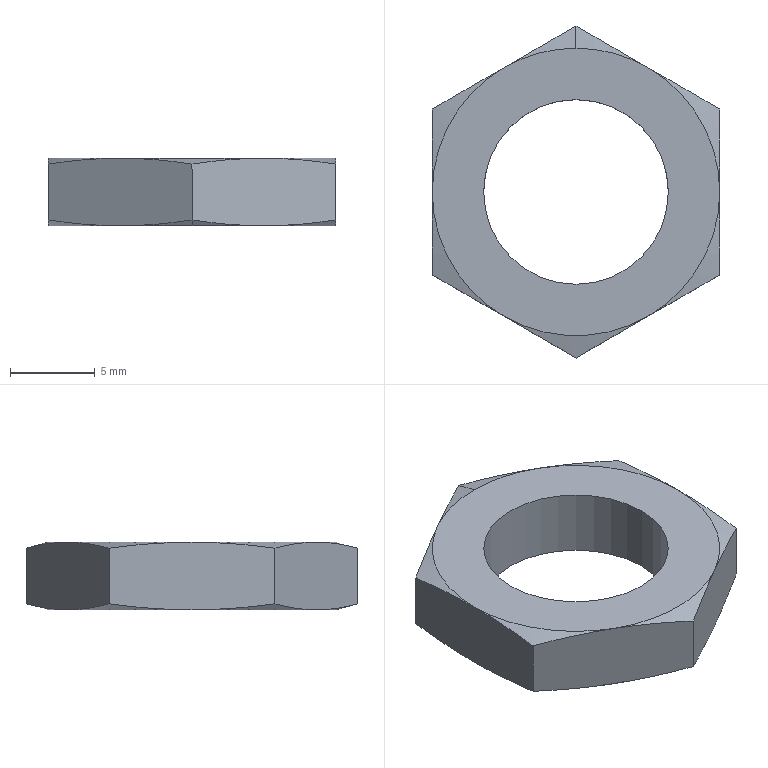Part | SolidWorks | features BaseBody 1 | 1 solid | 24 faces | box 17 x 19.63 x 4 mm | volume 621.409 mm3 | cone 14 | plane 8 | cylinder 2 | commonest cylinder face diameters 10.92 x2
STEP:
#1=CARTESIAN_POINT('',(5.46,0.,-4.));
#2=VERTEX_POINT('',#1);
#3=CARTESIAN_POINT('',(-5.46,0.,-4.));
#4=VERTEX_POINT('',#3);
#5=CARTESIAN_POINT('',(0.,0.,-4.));
#6=DIRECTION('',(0.,0.,-1.));
#7=DIRECTION('',(1.,0.,0.));
#8=AXIS2_PLACEMENT_3D('',#5,#6,#7);
#9=CIRCLE('',#8,5.46);
#10=EDGE_CURVE('',#2,#4,#9,.T.);
#11=ORIENTED_EDGE('',*,*,#10,.T.);
#12=CARTESIAN_POINT('',(-5.46,0.,0.));
#13=VERTEX_POINT('',#12);
#14=CARTESIAN_POINT('',(-5.46,0.,-4.));
#15=DIRECTION('',(0.,0.,1.));
#16=VECTOR('',#15,1000.);
#17=LINE('',#14,#16);
#18=EDGE_CURVE('',#4,#13,#17,.T.);
#19=ORIENTED_EDGE('',*,*,#18,.T.);
#20=CARTESIAN_POINT('',(5.46,0.,0.));
#21=VERTEX_POINT('',#20);
#22=CARTESIAN_POINT('',(0.,0.,0.));
#23=DIRECTION('',(0.,0.,-1.));
#24=DIRECTION('',(1.,0.,0.));
#25=AXIS2_PLACEMENT_3D('',#22,#23,#24);
#26=CIRCLE('',#25,5.46);
#27=EDGE_CURVE('',#21,#13,#26,.T.);
#28=ORIENTED_EDGE('',*,*,#27,.F.);
#29=CARTESIAN_POINT('',(5.46,0.,-4.));
#30=DIRECTION('',(0.,0.,1.));
#31=VECTOR('',#30,1000.);
#32=LINE('',#29,#31);
#33=EDGE_CURVE('',#2,#21,#32,.T.);
#34=ORIENTED_EDGE('',*,*,#33,.F.);
#35=EDGE_LOOP('',(#11,#19,#28,#34));
#36=FACE_OUTER_BOUND('',#35,.T.);
#37=CARTESIAN_POINT('',(0.,0.,-4.));
#38=DIRECTION('',(0.,0.,1.));
#39=DIRECTION('',(1.,0.,0.));
#40=AXIS2_PLACEMENT_3D('',#37,#38,#39);
#41=CYLINDRICAL_SURFACE('',#40,5.46);
#42=ADVANCED_FACE('',(#36),#41,.F.);
#43=CARTESIAN_POINT('',(-4.25,-7.361,-4.));
#44=VERTEX_POINT('',#43);
#45=CARTESIAN_POINT('',(0.,-8.5,-4.));
#46=VERTEX_POINT('',#45);
#47=CARTESIAN_POINT('',(0.,0.,-4.));
#48=DIRECTION('',(0.,0.,1.));
#49=DIRECTION('',(0.,-1.,0.));
#50=AXIS2_PLACEMENT_3D('',#47,#48,#49);
#51=CIRCLE('',#50,8.5);
#52=EDGE_CURVE('',#44,#46,#51,.T.);
#53=ORIENTED_EDGE('',*,*,#52,.T.);
#54=CARTESIAN_POINT('',(0.000000017,-9.815,-3.648));
#55=VERTEX_POINT('',#54);
#56=CARTESIAN_POINT('',(0.,-9.823,-3.646));
#57=DIRECTION('',(0.,-0.9659,0.2588));
#58=VECTOR('',#57,1000.);
#59=LINE('',#56,#58);
#60=EDGE_CURVE('',#46,#55,#59,.T.);
#61=ORIENTED_EDGE('',*,*,#60,.T.);
#62=CARTESIAN_POINT('',(0.000000017,-9.815,-3.648));
#63=CARTESIAN_POINT('',(-1.41,-9.001,-3.866));
#64=CARTESIAN_POINT('',(-2.826,-8.183,-4.));
#65=CARTESIAN_POINT('',(-4.25,-7.361,-4.));
#66=B_SPLINE_CURVE_WITH_KNOTS('',3,(#62,#63,#64,#65),.UNSPECIFIED.,.F.,.F.,(4,4),(0.,0.00492),.UNSPECIFIED.);
#67=EDGE_CURVE('',#55,#44,#66,.T.);
#68=ORIENTED_EDGE('',*,*,#67,.T.);
#69=EDGE_LOOP('',(#53,#61,#68));
#70=FACE_OUTER_BOUND('',#69,.T.);
#71=CARTESIAN_POINT('',(0.,0.,-3.646));
#72=DIRECTION('',(0.,0.,1.));
#73=DIRECTION('',(0.,-1.,0.));
#74=AXIS2_PLACEMENT_3D('',#71,#72,#73);
#75=CONICAL_SURFACE('',#74,9.823,1.309);
#76=ADVANCED_FACE('',(#70),#75,.T.);
#77=CARTESIAN_POINT('',(0.,8.5,0.));
#78=VERTEX_POINT('',#77);
#79=CARTESIAN_POINT('',(-4.25,7.361,0.));
#80=VERTEX_POINT('',#79);
#81=CARTESIAN_POINT('',(0.,0.,0.));
#82=DIRECTION('',(0.,0.,1.));
#83=DIRECTION('',(0.,1.,0.));
#84=AXIS2_PLACEMENT_3D('',#81,#82,#83);
#85=CIRCLE('',#84,8.5);
#86=EDGE_CURVE('',#78,#80,#85,.T.);
#87=ORIENTED_EDGE('',*,*,#86,.F.);
#88=CARTESIAN_POINT('',(0.,9.815,-0.3523));
#89=VERTEX_POINT('',#88);
#90=CARTESIAN_POINT('',(0.,9.823,-0.3545));
#91=DIRECTION('',(0.,0.9659,-0.2588));
#92=VECTOR('',#91,1000.);
#93=LINE('',#90,#92);
#94=EDGE_CURVE('',#78,#89,#93,.T.);
#95=ORIENTED_EDGE('',*,*,#94,.T.);
#96=CARTESIAN_POINT('',(-4.25,7.361,0.));
#97=CARTESIAN_POINT('',(-2.826,8.183,0.));
#98=CARTESIAN_POINT('',(-1.41,9.001,-0.1342));
#99=CARTESIAN_POINT('',(0.,9.815,-0.3523));
#100=B_SPLINE_CURVE_WITH_KNOTS('',3,(#96,#97,#98,#99),.UNSPECIFIED.,.F.,.F.,(4,4),(0.,0.00492),.UNSPECIFIED.);
#101=EDGE_CURVE('',#80,#89,#100,.T.);
#102=ORIENTED_EDGE('',*,*,#101,.F.);
#103=EDGE_LOOP('',(#87,#95,#102));
#104=FACE_OUTER_BOUND('',#103,.T.);
#105=CARTESIAN_POINT('',(0.,0.,-0.3545));
#106=DIRECTION('',(0.,0.,-1.));
#107=DIRECTION('',(0.,1.,0.));
#108=AXIS2_PLACEMENT_3D('',#105,#106,#107);
#109=CONICAL_SURFACE('',#108,9.823,1.309);
#110=ADVANCED_FACE('',(#104),#109,.T.);
#111=ORIENTED_EDGE('',*,*,#10,.F.);
#112=CARTESIAN_POINT('',(0.,0.,-4.));
#113=DIRECTION('',(0.,0.,-1.));
#114=DIRECTION('',(1.,0.,0.));
#115=AXIS2_PLACEMENT_3D('',#112,#113,#114);
#116=CIRCLE('',#115,5.46);
#117=EDGE_CURVE('',#4,#2,#116,.T.);
#118=ORIENTED_EDGE('',*,*,#117,.F.);
#119=EDGE_LOOP('',(#111,#118));
#120=FACE_BOUND('',#119,.T.);
#121=ORIENTED_EDGE('',*,*,#52,.F.);
#122=CARTESIAN_POINT('',(-8.5,0.,-4.));
#123=VERTEX_POINT('',#122);
#124=CARTESIAN_POINT('',(0.,0.,-4.));
#125=DIRECTION('',(0.,0.,1.));
#126=DIRECTION('',(0.,-1.,0.));
#127=AXIS2_PLACEMENT_3D('',#124,#125,#126);
#128=CIRCLE('',#127,8.5);
#129=EDGE_CURVE('',#123,#44,#128,.T.);
#130=ORIENTED_EDGE('',*,*,#129,.F.);
#131=CARTESIAN_POINT('',(-4.25,7.361,-4.));
#132=VERTEX_POINT('',#131);
#133=CARTESIAN_POINT('',(0.,0.,-4.));
#134=DIRECTION('',(0.,0.,1.));
#135=DIRECTION('',(1.,0.,0.));
#136=AXIS2_PLACEMENT_3D('',#133,#134,#135);
#137=CIRCLE('',#136,8.5);
#138=EDGE_CURVE('',#132,#123,#137,.T.);
#139=ORIENTED_EDGE('',*,*,#138,.F.);
#140=CARTESIAN_POINT('',(4.25,7.361,-4.));
#141=VERTEX_POINT('',#140);
#142=CARTESIAN_POINT('',(0.,0.,-4.));
#143=DIRECTION('',(0.,0.,1.));
#144=DIRECTION('',(1.,0.,0.));
#145=AXIS2_PLACEMENT_3D('',#142,#143,#144);
#146=CIRCLE('',#145,8.5);
#147=EDGE_CURVE('',#141,#132,#146,.T.);
#148=ORIENTED_EDGE('',*,*,#147,.F.);
#149=CARTESIAN_POINT('',(8.5,0.,-4.));
#150=VERTEX_POINT('',#149);
#151=CARTESIAN_POINT('',(0.,0.,-4.));
#152=DIRECTION('',(0.,0.,1.));
#153=DIRECTION('',(0.,-1.,0.));
#154=AXIS2_PLACEMENT_3D('',#151,#152,#153);
#155=CIRCLE('',#154,8.5);
#156=EDGE_CURVE('',#150,#141,#155,.T.);
#157=ORIENTED_EDGE('',*,*,#156,.F.);
#158=CARTESIAN_POINT('',(4.25,-7.361,-4.));
#159=VERTEX_POINT('',#158);
#160=CARTESIAN_POINT('',(0.,0.,-4.));
#161=DIRECTION('',(0.,0.,1.));
#162=DIRECTION('',(0.,-1.,0.));
#163=AXIS2_PLACEMENT_3D('',#160,#161,#162);
#164=CIRCLE('',#163,8.5);
#165=EDGE_CURVE('',#159,#150,#164,.T.);
#166=ORIENTED_EDGE('',*,*,#165,.F.);
#167=CARTESIAN_POINT('',(0.,0.,-4.));
#168=DIRECTION('',(0.,0.,1.));
#169=DIRECTION('',(0.,-1.,0.));
#170=AXIS2_PLACEMENT_3D('',#167,#168,#169);
#171=CIRCLE('',#170,8.5);
#172=EDGE_CURVE('',#46,#159,#171,.T.);
#173=ORIENTED_EDGE('',*,*,#172,.F.);
#174=EDGE_LOOP('',(#121,#130,#139,#148,#157,#166,#173));
#175=FACE_OUTER_BOUND('',#174,.T.);
#176=CARTESIAN_POINT('',(-17.,0.,-4.));
#177=DIRECTION('',(0.,0.,1.));
#178=DIRECTION('',(1.,0.,0.));
#179=AXIS2_PLACEMENT_3D('',#176,#177,#178);
#180=PLANE('',#179);
#181=ADVANCED_FACE('',(#120,#175),#180,.F.);
#182=ORIENTED_EDGE('',*,*,#18,.F.);
#183=ORIENTED_EDGE('',*,*,#117,.T.);
#184=ORIENTED_EDGE('',*,*,#33,.T.);
#185=CARTESIAN_POINT('',(0.,0.,0.));
#186=DIRECTION('',(0.,0.,-1.));
#187=DIRECTION('',(1.,0.,0.));
#188=AXIS2_PLACEMENT_3D('',#185,#186,#187);
#189=CIRCLE('',#188,5.46);
#190=EDGE_CURVE('',#13,#21,#189,.T.);
#191=ORIENTED_EDGE('',*,*,#190,.F.);
#192=EDGE_LOOP('',(#182,#183,#184,#191));
#193=FACE_OUTER_BOUND('',#192,.T.);
#194=CARTESIAN_POINT('',(0.,0.,-4.));
#195=DIRECTION('',(0.,0.,1.));
#196=DIRECTION('',(1.,0.,0.));
#197=AXIS2_PLACEMENT_3D('',#194,#195,#196);
#198=CYLINDRICAL_SURFACE('',#197,5.46);
#199=ADVANCED_FACE('',(#193),#198,.F.);
#200=CARTESIAN_POINT('',(8.5,-4.907,-3.648));
#201=VERTEX_POINT('',#200);
#202=CARTESIAN_POINT('',(8.5,0.,-4.));
#203=CARTESIAN_POINT('',(8.5,-1.644,-4.));
#204=CARTESIAN_POINT('',(8.5,-3.279,-3.866));
#205=CARTESIAN_POINT('',(8.5,-4.907,-3.648));
#206=B_SPLINE_CURVE_WITH_KNOTS('',3,(#202,#203,#204,#205),.UNSPECIFIED.,.F.,.F.,(4,4),(0.,0.00492),.UNSPECIFIED.);
#207=EDGE_CURVE('',#150,#201,#206,.T.);
#208=ORIENTED_EDGE('',*,*,#207,.T.);
#209=CARTESIAN_POINT('',(8.5,-4.907,-3.648));
#210=CARTESIAN_POINT('',(7.09,-5.722,-3.866));
#211=CARTESIAN_POINT('',(5.674,-6.539,-4.));
#212=CARTESIAN_POINT('',(4.25,-7.361,-4.));
#213=B_SPLINE_CURVE_WITH_KNOTS('',3,(#209,#210,#211,#212),.UNSPECIFIED.,.F.,.F.,(4,4),(0.,0.00492),.UNSPECIFIED.);
#214=EDGE_CURVE('',#201,#159,#213,.T.);
#215=ORIENTED_EDGE('',*,*,#214,.T.);
#216=ORIENTED_EDGE('',*,*,#165,.T.);
#217=EDGE_LOOP('',(#208,#215,#216));
#218=FACE_OUTER_BOUND('',#217,.T.);
#219=CARTESIAN_POINT('',(0.,0.,-3.646));
#220=DIRECTION('',(0.,0.,1.));
#221=DIRECTION('',(0.,-1.,0.));
#222=AXIS2_PLACEMENT_3D('',#219,#220,#221);
#223=CONICAL_SURFACE('',#222,9.823,1.309);
#224=ADVANCED_FACE('',(#218),#223,.T.);
#225=ORIENTED_EDGE('',*,*,#60,.F.);
#226=ORIENTED_EDGE('',*,*,#172,.T.);
#227=CARTESIAN_POINT('',(4.25,-7.361,-4.));
#228=CARTESIAN_POINT('',(2.826,-8.183,-4.));
#229=CARTESIAN_POINT('',(1.41,-9.001,-3.866));
#230=CARTESIAN_POINT('',(0.000000017,-9.815,-3.648));
#231=B_SPLINE_CURVE_WITH_KNOTS('',3,(#227,#228,#229,#230),.UNSPECIFIED.,.F.,.F.,(4,4),(0.,0.00492),.UNSPECIFIED.);
#232=EDGE_CURVE('',#159,#55,#231,.T.);
#233=ORIENTED_EDGE('',*,*,#232,.T.);
#234=EDGE_LOOP('',(#225,#226,#233));
#235=FACE_OUTER_BOUND('',#234,.T.);
#236=CARTESIAN_POINT('',(0.,0.,-3.646));
#237=DIRECTION('',(0.,0.,1.));
#238=DIRECTION('',(0.,-1.,0.));
#239=AXIS2_PLACEMENT_3D('',#236,#237,#238);
#240=CONICAL_SURFACE('',#239,9.823,1.309);
#241=ADVANCED_FACE('',(#235),#240,.T.);
#242=ORIENTED_EDGE('',*,*,#129,.T.);
#243=CARTESIAN_POINT('',(-8.5,-4.907,-3.648));
#244=VERTEX_POINT('',#243);
#245=CARTESIAN_POINT('',(-4.25,-7.361,-4.));
#246=CARTESIAN_POINT('',(-5.674,-6.539,-4.));
#247=CARTESIAN_POINT('',(-7.09,-5.722,-3.866));
#248=CARTESIAN_POINT('',(-8.5,-4.907,-3.648));
#249=B_SPLINE_CURVE_WITH_KNOTS('',3,(#245,#246,#247,#248),.UNSPECIFIED.,.F.,.F.,(4,4),(0.,0.00492),.UNSPECIFIED.);
#250=EDGE_CURVE('',#44,#244,#249,.T.);
#251=ORIENTED_EDGE('',*,*,#250,.T.);
#252=CARTESIAN_POINT('',(-8.5,-4.907,-3.648));
#253=CARTESIAN_POINT('',(-8.5,-3.279,-3.866));
#254=CARTESIAN_POINT('',(-8.5,-1.644,-4.));
#255=CARTESIAN_POINT('',(-8.5,0.,-4.));
#256=B_SPLINE_CURVE_WITH_KNOTS('',3,(#252,#253,#254,#255),.UNSPECIFIED.,.F.,.F.,(4,4),(0.,0.00492),.UNSPECIFIED.);
#257=EDGE_CURVE('',#244,#123,#256,.T.);
#258=ORIENTED_EDGE('',*,*,#257,.T.);
#259=EDGE_LOOP('',(#242,#251,#258));
#260=FACE_OUTER_BOUND('',#259,.T.);
#261=CARTESIAN_POINT('',(0.,0.,-3.646));
#262=DIRECTION('',(0.,0.,1.));
#263=DIRECTION('',(0.,-1.,0.));
#264=AXIS2_PLACEMENT_3D('',#261,#262,#263);
#265=CONICAL_SURFACE('',#264,9.823,1.309);
#266=ADVANCED_FACE('',(#260),#265,.T.);
#267=CARTESIAN_POINT('',(-8.5,4.907,-3.648));
#268=VERTEX_POINT('',#267);
#269=CARTESIAN_POINT('',(-8.5,0.,-4.));
#270=CARTESIAN_POINT('',(-8.5,1.644,-4.));
#271=CARTESIAN_POINT('',(-8.5,3.279,-3.866));
#272=CARTESIAN_POINT('',(-8.5,4.907,-3.648));
#273=B_SPLINE_CURVE_WITH_KNOTS('',3,(#269,#270,#271,#272),.UNSPECIFIED.,.F.,.F.,(4,4),(0.,0.00492),.UNSPECIFIED.);
#274=EDGE_CURVE('',#123,#268,#273,.T.);
#275=ORIENTED_EDGE('',*,*,#274,.T.);
#276=CARTESIAN_POINT('',(-8.5,4.907,-3.648));
#277=CARTESIAN_POINT('',(-7.09,5.722,-3.866));
#278=CARTESIAN_POINT('',(-5.674,6.539,-4.));
#279=CARTESIAN_POINT('',(-4.25,7.361,-4.));
#280=B_SPLINE_CURVE_WITH_KNOTS('',3,(#276,#277,#278,#279),.UNSPECIFIED.,.F.,.F.,(4,4),(0.,0.00492),.UNSPECIFIED.);
#281=EDGE_CURVE('',#268,#132,#280,.T.);
#282=ORIENTED_EDGE('',*,*,#281,.T.);
#283=ORIENTED_EDGE('',*,*,#138,.T.);
#284=EDGE_LOOP('',(#275,#282,#283));
#285=FACE_OUTER_BOUND('',#284,.T.);
#286=CARTESIAN_POINT('',(0.,0.,-3.646));
#287=DIRECTION('',(0.,0.,1.));
#288=DIRECTION('',(1.,0.,0.));
#289=AXIS2_PLACEMENT_3D('',#286,#287,#288);
#290=CONICAL_SURFACE('',#289,9.823,1.309);
#291=ADVANCED_FACE('',(#285),#290,.T.);
#292=ORIENTED_EDGE('',*,*,#147,.T.);
#293=CARTESIAN_POINT('',(0.000000022,9.815,-3.648));
#294=VERTEX_POINT('',#293);
#295=CARTESIAN_POINT('',(-4.25,7.361,-4.));
#296=CARTESIAN_POINT('',(-2.826,8.183,-4.));
#297=CARTESIAN_POINT('',(-1.41,9.001,-3.866));
#298=CARTESIAN_POINT('',(0.000000022,9.815,-3.648));
#299=B_SPLINE_CURVE_WITH_KNOTS('',3,(#295,#296,#297,#298),.UNSPECIFIED.,.F.,.F.,(4,4),(0.,0.00492),.UNSPECIFIED.);
#300=EDGE_CURVE('',#132,#294,#299,.T.);
#301=ORIENTED_EDGE('',*,*,#300,.T.);
#302=CARTESIAN_POINT('',(0.000000022,9.815,-3.648));
#303=CARTESIAN_POINT('',(1.41,9.001,-3.866));
#304=CARTESIAN_POINT('',(2.826,8.183,-4.));
#305=CARTESIAN_POINT('',(4.25,7.361,-4.));
#306=B_SPLINE_CURVE_WITH_KNOTS('',3,(#302,#303,#304,#305),.UNSPECIFIED.,.F.,.F.,(4,4),(0.,0.00492),.UNSPECIFIED.);
#307=EDGE_CURVE('',#294,#141,#306,.T.);
#308=ORIENTED_EDGE('',*,*,#307,.T.);
#309=EDGE_LOOP('',(#292,#301,#308));
#310=FACE_OUTER_BOUND('',#309,.T.);
#311=CARTESIAN_POINT('',(0.,0.,-3.646));
#312=DIRECTION('',(0.,0.,1.));
#313=DIRECTION('',(1.,0.,0.));
#314=AXIS2_PLACEMENT_3D('',#311,#312,#313);
#315=CONICAL_SURFACE('',#314,9.823,1.309);
#316=ADVANCED_FACE('',(#310),#315,.T.);
#317=ORIENTED_EDGE('',*,*,#156,.T.);
#318=CARTESIAN_POINT('',(8.5,4.907,-3.648));
#319=VERTEX_POINT('',#318);
#320=CARTESIAN_POINT('',(4.25,7.361,-4.));
#321=CARTESIAN_POINT('',(5.674,6.539,-4.));
#322=CARTESIAN_POINT('',(7.09,5.722,-3.866));
#323=CARTESIAN_POINT('',(8.5,4.907,-3.648));
#324=B_SPLINE_CURVE_WITH_KNOTS('',3,(#320,#321,#322,#323),.UNSPECIFIED.,.F.,.F.,(4,4),(0.,0.00492),.UNSPECIFIED.);
#325=EDGE_CURVE('',#141,#319,#324,.T.);
#326=ORIENTED_EDGE('',*,*,#325,.T.);
#327=CARTESIAN_POINT('',(8.5,4.907,-3.648));
#328=CARTESIAN_POINT('',(8.5,3.279,-3.866));
#329=CARTESIAN_POINT('',(8.5,1.644,-4.));
#330=CARTESIAN_POINT('',(8.5,0.,-4.));
#331=B_SPLINE_CURVE_WITH_KNOTS('',3,(#327,#328,#329,#330),.UNSPECIFIED.,.F.,.F.,(4,4),(0.,0.00492),.UNSPECIFIED.);
#332=EDGE_CURVE('',#319,#150,#331,.T.);
#333=ORIENTED_EDGE('',*,*,#332,.T.);
#334=EDGE_LOOP('',(#317,#326,#333));
#335=FACE_OUTER_BOUND('',#334,.T.);
#336=CARTESIAN_POINT('',(0.,0.,-3.646));
#337=DIRECTION('',(0.,0.,1.));
#338=DIRECTION('',(0.,-1.,0.));
#339=AXIS2_PLACEMENT_3D('',#336,#337,#338);
#340=CONICAL_SURFACE('',#339,9.823,1.309);
#341=ADVANCED_FACE('',(#335),#340,.T.);
#342=ORIENTED_EDGE('',*,*,#27,.T.);
#343=ORIENTED_EDGE('',*,*,#190,.T.);
#344=EDGE_LOOP('',(#342,#343));
#345=FACE_BOUND('',#344,.T.);
#346=CARTESIAN_POINT('',(4.25,7.361,0.));
#347=VERTEX_POINT('',#346);
#348=CARTESIAN_POINT('',(0.,0.,0.));
#349=DIRECTION('',(0.,0.,1.));
#350=DIRECTION('',(0.,1.,0.));
#351=AXIS2_PLACEMENT_3D('',#348,#349,#350);
#352=CIRCLE('',#351,8.5);
#353=EDGE_CURVE('',#347,#78,#352,.T.);
#354=ORIENTED_EDGE('',*,*,#353,.T.);
#355=ORIENTED_EDGE('',*,*,#86,.T.);
#356=CARTESIAN_POINT('',(-8.5,0.,0.));
#357=VERTEX_POINT('',#356);
#358=CARTESIAN_POINT('',(0.,0.,0.));
#359=DIRECTION('',(0.,0.,1.));
#360=DIRECTION('',(-1.,0.,0.));
#361=AXIS2_PLACEMENT_3D('',#358,#359,#360);
#362=CIRCLE('',#361,8.5);
#363=EDGE_CURVE('',#80,#357,#362,.T.);
#364=ORIENTED_EDGE('',*,*,#363,.T.);
#365=CARTESIAN_POINT('',(-4.25,-7.361,0.));
#366=VERTEX_POINT('',#365);
#367=CARTESIAN_POINT('',(0.,0.,0.));
#368=DIRECTION('',(0.,0.,1.));
#369=DIRECTION('',(-1.,0.,0.));
#370=AXIS2_PLACEMENT_3D('',#367,#368,#369);
#371=CIRCLE('',#370,8.5);
#372=EDGE_CURVE('',#357,#366,#371,.T.);
#373=ORIENTED_EDGE('',*,*,#372,.T.);
#374=CARTESIAN_POINT('',(4.25,-7.361,0.));
#375=VERTEX_POINT('',#374);
#376=CARTESIAN_POINT('',(0.,0.,0.));
#377=DIRECTION('',(0.,0.,1.));
#378=DIRECTION('',(-1.,0.,0.));
#379=AXIS2_PLACEMENT_3D('',#376,#377,#378);
#380=CIRCLE('',#379,8.5);
#381=EDGE_CURVE('',#366,#375,#380,.T.);
#382=ORIENTED_EDGE('',*,*,#381,.T.);
#383=CARTESIAN_POINT('',(8.5,0.,0.));
#384=VERTEX_POINT('',#383);
#385=CARTESIAN_POINT('',(0.,0.,0.));
#386=DIRECTION('',(0.,0.,1.));
#387=DIRECTION('',(0.,1.,0.));
#388=AXIS2_PLACEMENT_3D('',#385,#386,#387);
#389=CIRCLE('',#388,8.5);
#390=EDGE_CURVE('',#375,#384,#389,.T.);
#391=ORIENTED_EDGE('',*,*,#390,.T.);
#392=CARTESIAN_POINT('',(0.,0.,0.));
#393=DIRECTION('',(0.,0.,1.));
#394=DIRECTION('',(-1.,0.,0.));
#395=AXIS2_PLACEMENT_3D('',#392,#393,#394);
#396=CIRCLE('',#395,8.5);
#397=EDGE_CURVE('',#384,#347,#396,.T.);
#398=ORIENTED_EDGE('',*,*,#397,.T.);
#399=EDGE_LOOP('',(#354,#355,#364,#373,#382,#391,#398));
#400=FACE_OUTER_BOUND('',#399,.T.);
#401=CARTESIAN_POINT('',(-17.,0.,0.));
#402=DIRECTION('',(0.,0.,1.));
#403=DIRECTION('',(1.,0.,0.));
#404=AXIS2_PLACEMENT_3D('',#401,#402,#403);
#405=PLANE('',#404);
#406=ADVANCED_FACE('',(#345,#400),#405,.T.);
#407=CARTESIAN_POINT('',(0.,-9.815,-0.3523));
#408=VERTEX_POINT('',#407);
#409=CARTESIAN_POINT('',(4.25,-7.361,0.));
#410=CARTESIAN_POINT('',(2.826,-8.183,0.));
#411=CARTESIAN_POINT('',(1.41,-9.001,-0.1342));
#412=CARTESIAN_POINT('',(0.,-9.815,-0.3523));
#413=B_SPLINE_CURVE_WITH_KNOTS('',3,(#409,#410,#411,#412),.UNSPECIFIED.,.F.,.F.,(4,4),(0.,0.00492),.UNSPECIFIED.);
#414=EDGE_CURVE('',#375,#408,#413,.T.);
#415=ORIENTED_EDGE('',*,*,#414,.T.);
#416=CARTESIAN_POINT('',(0.,-9.815,-4.));
#417=DIRECTION('',(0.,0.,-1.));
#418=VECTOR('',#417,1000.);
#419=LINE('',#416,#418);
#420=EDGE_CURVE('',#408,#55,#419,.T.);
#421=ORIENTED_EDGE('',*,*,#420,.T.);
#422=ORIENTED_EDGE('',*,*,#232,.F.);
#423=ORIENTED_EDGE('',*,*,#214,.F.);
#424=CARTESIAN_POINT('',(8.5,-4.907,-0.3523));
#425=VERTEX_POINT('',#424);
#426=CARTESIAN_POINT('',(8.5,-4.907,-4.));
#427=DIRECTION('',(0.,0.,1.));
#428=VECTOR('',#427,1000.);
#429=LINE('',#426,#428);
#430=EDGE_CURVE('',#201,#425,#429,.T.);
#431=ORIENTED_EDGE('',*,*,#430,.T.);
#432=CARTESIAN_POINT('',(8.5,-4.907,-0.3523));
#433=CARTESIAN_POINT('',(7.09,-5.722,-0.1342));
#434=CARTESIAN_POINT('',(5.674,-6.539,0.));
#435=CARTESIAN_POINT('',(4.25,-7.361,0.));
#436=B_SPLINE_CURVE_WITH_KNOTS('',3,(#432,#433,#434,#435),.UNSPECIFIED.,.F.,.F.,(4,4),(0.,0.00492),.UNSPECIFIED.);
#437=EDGE_CURVE('',#425,#375,#436,.T.);
#438=ORIENTED_EDGE('',*,*,#437,.T.);
#439=EDGE_LOOP('',(#415,#421,#422,#423,#431,#438));
#440=FACE_OUTER_BOUND('',#439,.T.);
#441=CARTESIAN_POINT('',(0.,-9.815,-4.));
#442=DIRECTION('',(0.5,-0.866,0.));
#443=DIRECTION('',(0.866,0.5,0.));
#444=AXIS2_PLACEMENT_3D('',#441,#442,#443);
#445=PLANE('',#444);
#446=ADVANCED_FACE('',(#440),#445,.T.);
#447=ORIENTED_EDGE('',*,*,#207,.F.);
#448=ORIENTED_EDGE('',*,*,#332,.F.);
#449=CARTESIAN_POINT('',(8.5,4.907,-0.3523));
#450=VERTEX_POINT('',#449);
#451=CARTESIAN_POINT('',(8.5,4.907,-4.));
#452=DIRECTION('',(0.,0.,-1.));
#453=VECTOR('',#452,1000.);
#454=LINE('',#451,#453);
#455=EDGE_CURVE('',#450,#319,#454,.T.);
#456=ORIENTED_EDGE('',*,*,#455,.F.);
#457=CARTESIAN_POINT('',(8.5,0.,0.));
#458=CARTESIAN_POINT('',(8.5,1.644,0.));
#459=CARTESIAN_POINT('',(8.5,3.279,-0.1342));
#460=CARTESIAN_POINT('',(8.5,4.907,-0.3523));
#461=B_SPLINE_CURVE_WITH_KNOTS('',3,(#457,#458,#459,#460),.UNSPECIFIED.,.F.,.F.,(4,4),(0.,0.00492),.UNSPECIFIED.);
#462=EDGE_CURVE('',#384,#450,#461,.T.);
#463=ORIENTED_EDGE('',*,*,#462,.F.);
#464=CARTESIAN_POINT('',(8.5,-4.907,-0.3523));
#465=CARTESIAN_POINT('',(8.5,-3.279,-0.1342));
#466=CARTESIAN_POINT('',(8.5,-1.644,0.));
#467=CARTESIAN_POINT('',(8.5,0.,0.));
#468=B_SPLINE_CURVE_WITH_KNOTS('',3,(#464,#465,#466,#467),.UNSPECIFIED.,.F.,.F.,(4,4),(0.,0.00492),.UNSPECIFIED.);
#469=EDGE_CURVE('',#425,#384,#468,.T.);
#470=ORIENTED_EDGE('',*,*,#469,.F.);
#471=ORIENTED_EDGE('',*,*,#430,.F.);
#472=EDGE_LOOP('',(#447,#448,#456,#463,#470,#471));
#473=FACE_OUTER_BOUND('',#472,.T.);
#474=CARTESIAN_POINT('',(8.5,4.907,-4.));
#475=DIRECTION('',(-1.,0.,0.));
#476=DIRECTION('',(0.,0.,1.));
#477=AXIS2_PLACEMENT_3D('',#474,#475,#476);
#478=PLANE('',#477);
#479=ADVANCED_FACE('',(#473),#478,.F.);
#480=CARTESIAN_POINT('',(-8.5,-4.907,-0.3523));
#481=VERTEX_POINT('',#480);
#482=CARTESIAN_POINT('',(-4.25,-7.361,0.));
#483=CARTESIAN_POINT('',(-5.674,-6.539,0.));
#484=CARTESIAN_POINT('',(-7.09,-5.722,-0.1342));
#485=CARTESIAN_POINT('',(-8.5,-4.907,-0.3523));
#486=B_SPLINE_CURVE_WITH_KNOTS('',3,(#482,#483,#484,#485),.UNSPECIFIED.,.F.,.F.,(4,4),(0.,0.00492),.UNSPECIFIED.);
#487=EDGE_CURVE('',#366,#481,#486,.T.);
#488=ORIENTED_EDGE('',*,*,#487,.T.);
#489=CARTESIAN_POINT('',(-8.5,-4.907,-4.));
#490=DIRECTION('',(0.,0.,-1.));
#491=VECTOR('',#490,1000.);
#492=LINE('',#489,#491);
#493=EDGE_CURVE('',#481,#244,#492,.T.);
#494=ORIENTED_EDGE('',*,*,#493,.T.);
#495=ORIENTED_EDGE('',*,*,#250,.F.);
#496=ORIENTED_EDGE('',*,*,#67,.F.);
#497=ORIENTED_EDGE('',*,*,#420,.F.);
#498=CARTESIAN_POINT('',(0.,-9.815,-0.3523));
#499=CARTESIAN_POINT('',(-1.41,-9.001,-0.1342));
#500=CARTESIAN_POINT('',(-2.826,-8.183,0.));
#501=CARTESIAN_POINT('',(-4.25,-7.361,0.));
#502=B_SPLINE_CURVE_WITH_KNOTS('',3,(#498,#499,#500,#501),.UNSPECIFIED.,.F.,.F.,(4,4),(0.,0.00492),.UNSPECIFIED.);
#503=EDGE_CURVE('',#408,#366,#502,.T.);
#504=ORIENTED_EDGE('',*,*,#503,.T.);
#505=EDGE_LOOP('',(#488,#494,#495,#496,#497,#504));
#506=FACE_OUTER_BOUND('',#505,.T.);
#507=CARTESIAN_POINT('',(-8.5,-4.907,-4.));
#508=DIRECTION('',(-0.5,-0.866,0.));
#509=DIRECTION('',(0.866,-0.5,0.));
#510=AXIS2_PLACEMENT_3D('',#507,#508,#509);
#511=PLANE('',#510);
#512=ADVANCED_FACE('',(#506),#511,.T.);
#513=CARTESIAN_POINT('',(-8.5,4.907,-0.3523));
#514=VERTEX_POINT('',#513);
#515=CARTESIAN_POINT('',(-8.5,0.,0.));
#516=CARTESIAN_POINT('',(-8.5,1.644,0.));
#517=CARTESIAN_POINT('',(-8.5,3.279,-0.1342));
#518=CARTESIAN_POINT('',(-8.5,4.907,-0.3523));
#519=B_SPLINE_CURVE_WITH_KNOTS('',3,(#515,#516,#517,#518),.UNSPECIFIED.,.F.,.F.,(4,4),(0.,0.00492),.UNSPECIFIED.);
#520=EDGE_CURVE('',#357,#514,#519,.T.);
#521=ORIENTED_EDGE('',*,*,#520,.T.);
#522=CARTESIAN_POINT('',(-8.5,4.907,-4.));
#523=DIRECTION('',(0.,0.,-1.));
#524=VECTOR('',#523,1000.);
#525=LINE('',#522,#524);
#526=EDGE_CURVE('',#514,#268,#525,.T.);
#527=ORIENTED_EDGE('',*,*,#526,.T.);
#528=ORIENTED_EDGE('',*,*,#274,.F.);
#529=ORIENTED_EDGE('',*,*,#257,.F.);
#530=ORIENTED_EDGE('',*,*,#493,.F.);
#531=CARTESIAN_POINT('',(-8.5,-4.907,-0.3523));
#532=CARTESIAN_POINT('',(-8.5,-3.279,-0.1342));
#533=CARTESIAN_POINT('',(-8.5,-1.644,0.));
#534=CARTESIAN_POINT('',(-8.5,0.,0.));
#535=B_SPLINE_CURVE_WITH_KNOTS('',3,(#531,#532,#533,#534),.UNSPECIFIED.,.F.,.F.,(4,4),(0.,0.00492),.UNSPECIFIED.);
#536=EDGE_CURVE('',#481,#357,#535,.T.);
#537=ORIENTED_EDGE('',*,*,#536,.T.);
#538=EDGE_LOOP('',(#521,#527,#528,#529,#530,#537));
#539=FACE_OUTER_BOUND('',#538,.T.);
#540=CARTESIAN_POINT('',(-8.5,4.907,-4.));
#541=DIRECTION('',(-1.,0.,0.));
#542=DIRECTION('',(0.,0.,1.));
#543=AXIS2_PLACEMENT_3D('',#540,#541,#542);
#544=PLANE('',#543);
#545=ADVANCED_FACE('',(#539),#544,.T.);
#546=ORIENTED_EDGE('',*,*,#101,.T.);
#547=CARTESIAN_POINT('',(0.,9.815,-4.));
#548=DIRECTION('',(0.,0.,-1.));
#549=VECTOR('',#548,1000.);
#550=LINE('',#547,#549);
#551=EDGE_CURVE('',#89,#294,#550,.T.);
#552=ORIENTED_EDGE('',*,*,#551,.T.);
#553=ORIENTED_EDGE('',*,*,#300,.F.);
#554=ORIENTED_EDGE('',*,*,#281,.F.);
#555=ORIENTED_EDGE('',*,*,#526,.F.);
#556=CARTESIAN_POINT('',(-8.5,4.907,-0.3523));
#557=CARTESIAN_POINT('',(-7.09,5.722,-0.1342));
#558=CARTESIAN_POINT('',(-5.674,6.539,0.));
#559=CARTESIAN_POINT('',(-4.25,7.361,0.));
#560=B_SPLINE_CURVE_WITH_KNOTS('',3,(#556,#557,#558,#559),.UNSPECIFIED.,.F.,.F.,(4,4),(0.,0.00492),.UNSPECIFIED.);
#561=EDGE_CURVE('',#514,#80,#560,.T.);
#562=ORIENTED_EDGE('',*,*,#561,.T.);
#563=EDGE_LOOP('',(#546,#552,#553,#554,#555,#562));
#564=FACE_OUTER_BOUND('',#563,.T.);
#565=CARTESIAN_POINT('',(0.,9.815,-4.));
#566=DIRECTION('',(-0.5,0.866,0.));
#567=DIRECTION('',(-0.866,-0.5,0.));
#568=AXIS2_PLACEMENT_3D('',#565,#566,#567);
#569=PLANE('',#568);
#570=ADVANCED_FACE('',(#564),#569,.T.);
#571=CARTESIAN_POINT('',(4.25,7.361,0.));
#572=CARTESIAN_POINT('',(5.674,6.539,0.));
#573=CARTESIAN_POINT('',(7.09,5.722,-0.1342));
#574=CARTESIAN_POINT('',(8.5,4.907,-0.3523));
#575=B_SPLINE_CURVE_WITH_KNOTS('',3,(#571,#572,#573,#574),.UNSPECIFIED.,.F.,.F.,(4,4),(0.,0.00492),.UNSPECIFIED.);
#576=EDGE_CURVE('',#347,#450,#575,.T.);
#577=ORIENTED_EDGE('',*,*,#576,.T.);
#578=ORIENTED_EDGE('',*,*,#455,.T.);
#579=ORIENTED_EDGE('',*,*,#325,.F.);
#580=ORIENTED_EDGE('',*,*,#307,.F.);
#581=ORIENTED_EDGE('',*,*,#551,.F.);
#582=CARTESIAN_POINT('',(0.,9.815,-0.3523));
#583=CARTESIAN_POINT('',(1.41,9.001,-0.1342));
#584=CARTESIAN_POINT('',(2.826,8.183,0.));
#585=CARTESIAN_POINT('',(4.25,7.361,0.));
#586=B_SPLINE_CURVE_WITH_KNOTS('',3,(#582,#583,#584,#585),.UNSPECIFIED.,.F.,.F.,(4,4),(0.,0.00492),.UNSPECIFIED.);
#587=EDGE_CURVE('',#89,#347,#586,.T.);
#588=ORIENTED_EDGE('',*,*,#587,.T.);
#589=EDGE_LOOP('',(#577,#578,#579,#580,#581,#588));
#590=FACE_OUTER_BOUND('',#589,.T.);
#591=CARTESIAN_POINT('',(8.5,4.907,-4.));
#592=DIRECTION('',(0.5,0.866,0.));
#593=DIRECTION('',(-0.866,0.5,0.));
#594=AXIS2_PLACEMENT_3D('',#591,#592,#593);
#595=PLANE('',#594);
#596=ADVANCED_FACE('',(#590),#595,.T.);
#597=ORIENTED_EDGE('',*,*,#561,.F.);
#598=ORIENTED_EDGE('',*,*,#520,.F.);
#599=ORIENTED_EDGE('',*,*,#363,.F.);
#600=EDGE_LOOP('',(#597,#598,#599));
#601=FACE_OUTER_BOUND('',#600,.T.);
#602=CARTESIAN_POINT('',(0.,0.,-0.3545));
#603=DIRECTION('',(0.,0.,-1.));
#604=DIRECTION('',(-1.,0.,0.));
#605=AXIS2_PLACEMENT_3D('',#602,#603,#604);
#606=CONICAL_SURFACE('',#605,9.823,1.309);
#607=ADVANCED_FACE('',(#601),#606,.T.);
#608=ORIENTED_EDGE('',*,*,#94,.F.);
#609=ORIENTED_EDGE('',*,*,#353,.F.);
#610=ORIENTED_EDGE('',*,*,#587,.F.);
#611=EDGE_LOOP('',(#608,#609,#610));
#612=FACE_OUTER_BOUND('',#611,.T.);
#613=CARTESIAN_POINT('',(0.,0.,-0.3545));
#614=DIRECTION('',(0.,0.,-1.));
#615=DIRECTION('',(0.,1.,0.));
#616=AXIS2_PLACEMENT_3D('',#613,#614,#615);
#617=CONICAL_SURFACE('',#616,9.823,1.309);
#618=ADVANCED_FACE('',(#612),#617,.T.);
#619=ORIENTED_EDGE('',*,*,#576,.F.);
#620=ORIENTED_EDGE('',*,*,#397,.F.);
#621=ORIENTED_EDGE('',*,*,#462,.T.);
#622=EDGE_LOOP('',(#619,#620,#621));
#623=FACE_OUTER_BOUND('',#622,.T.);
#624=CARTESIAN_POINT('',(0.,0.,-0.3545));
#625=DIRECTION('',(0.,0.,-1.));
#626=DIRECTION('',(-1.,0.,0.));
#627=AXIS2_PLACEMENT_3D('',#624,#625,#626);
#628=CONICAL_SURFACE('',#627,9.823,1.309);
#629=ADVANCED_FACE('',(#623),#628,.T.);
#630=ORIENTED_EDGE('',*,*,#437,.F.);
#631=ORIENTED_EDGE('',*,*,#469,.T.);
#632=ORIENTED_EDGE('',*,*,#390,.F.);
#633=EDGE_LOOP('',(#630,#631,#632));
#634=FACE_OUTER_BOUND('',#633,.T.);
#635=CARTESIAN_POINT('',(0.,0.,-0.3545));
#636=DIRECTION('',(0.,0.,-1.));
#637=DIRECTION('',(0.,1.,0.));
#638=AXIS2_PLACEMENT_3D('',#635,#636,#637);
#639=CONICAL_SURFACE('',#638,9.823,1.309);
#640=ADVANCED_FACE('',(#634),#639,.T.);
#641=ORIENTED_EDGE('',*,*,#414,.F.);
#642=ORIENTED_EDGE('',*,*,#381,.F.);
#643=ORIENTED_EDGE('',*,*,#503,.F.);
#644=EDGE_LOOP('',(#641,#642,#643));
#645=FACE_OUTER_BOUND('',#644,.T.);
#646=CARTESIAN_POINT('',(0.,0.,-0.3545));
#647=DIRECTION('',(0.,0.,-1.));
#648=DIRECTION('',(-1.,0.,0.));
#649=AXIS2_PLACEMENT_3D('',#646,#647,#648);
#650=CONICAL_SURFACE('',#649,9.823,1.309);
#651=ADVANCED_FACE('',(#645),#650,.T.);
#652=ORIENTED_EDGE('',*,*,#487,.F.);
#653=ORIENTED_EDGE('',*,*,#372,.F.);
#654=ORIENTED_EDGE('',*,*,#536,.F.);
#655=EDGE_LOOP('',(#652,#653,#654));
#656=FACE_OUTER_BOUND('',#655,.T.);
#657=CARTESIAN_POINT('',(0.,0.,-0.3545));
#658=DIRECTION('',(0.,0.,-1.));
#659=DIRECTION('',(-1.,0.,0.));
#660=AXIS2_PLACEMENT_3D('',#657,#658,#659);
#661=CONICAL_SURFACE('',#660,9.823,1.309);
#662=ADVANCED_FACE('',(#656),#661,.T.);
#663=CLOSED_SHELL('',(#42,#76,#110,#181,#199,#224,#241,#266,#291,#316,#341,#406,#446,#479,#512,#545,#570,#596,#607,#618,#629,#640,#651,#662));
#664=MANIFOLD_SOLID_BREP('',#663);
#665=CARTESIAN_POINT('',(0.,0.,0.));
#666=DIRECTION('',(0.,0.,1.));
#667=DIRECTION('',(1.,0.,0.));
#668=AXIS2_PLACEMENT_3D('',#665,#666,#667);
#669=(LENGTH_UNIT()NAMED_UNIT(*)SI_UNIT(.MILLI.,.METRE.));
#670=UNCERTAINTY_MEASURE_WITH_UNIT(LENGTH_MEASURE(0.00001),#669,'','');
#671=(NAMED_UNIT(*)PLANE_ANGLE_UNIT()SI_UNIT($,.RADIAN.));
#672=(NAMED_UNIT(*)SI_UNIT($,.STERADIAN.)SOLID_ANGLE_UNIT());
#673=(GEOMETRIC_REPRESENTATION_CONTEXT(3)GLOBAL_UNCERTAINTY_ASSIGNED_CONTEXT((#670))GLOBAL_UNIT_ASSIGNED_CONTEXT((#669,#671,#672))REPRESENTATION_CONTEXT('',''));
#674=ADVANCED_BREP_SHAPE_REPRESENTATION('',(#664,#668),#673);